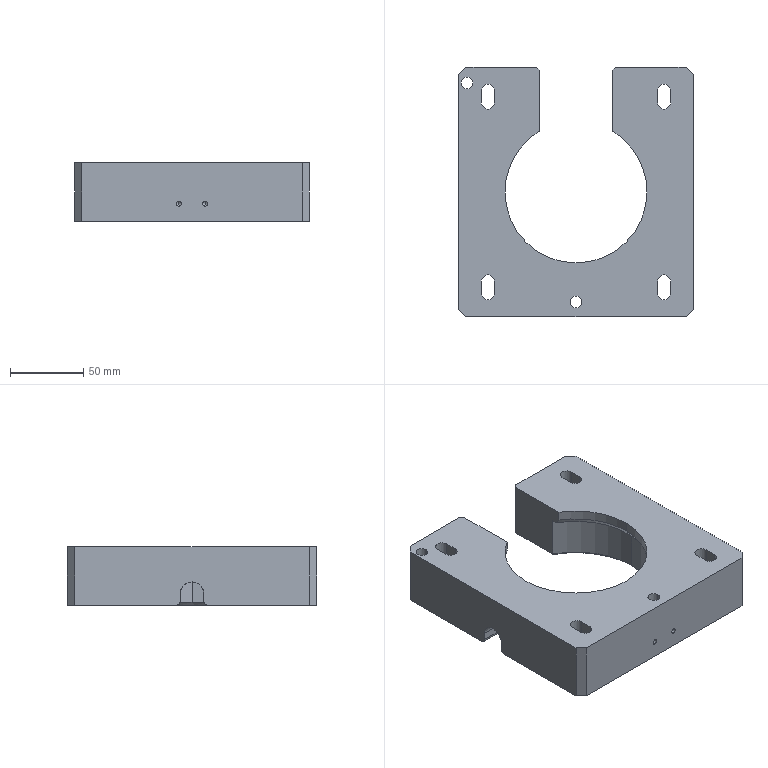Part | STEP file | PN_0008 Magazine clip fixing seat | 1 solid | 84 faces | box 160 x 170 x 40 mm | volume 624191 mm3 | plane 41 | cylinder 34 | cone 9 | commonest cylinder face diameters 9 x8 15 x8 3.3 x4 8 x4 96.75 x3 107.5 x3